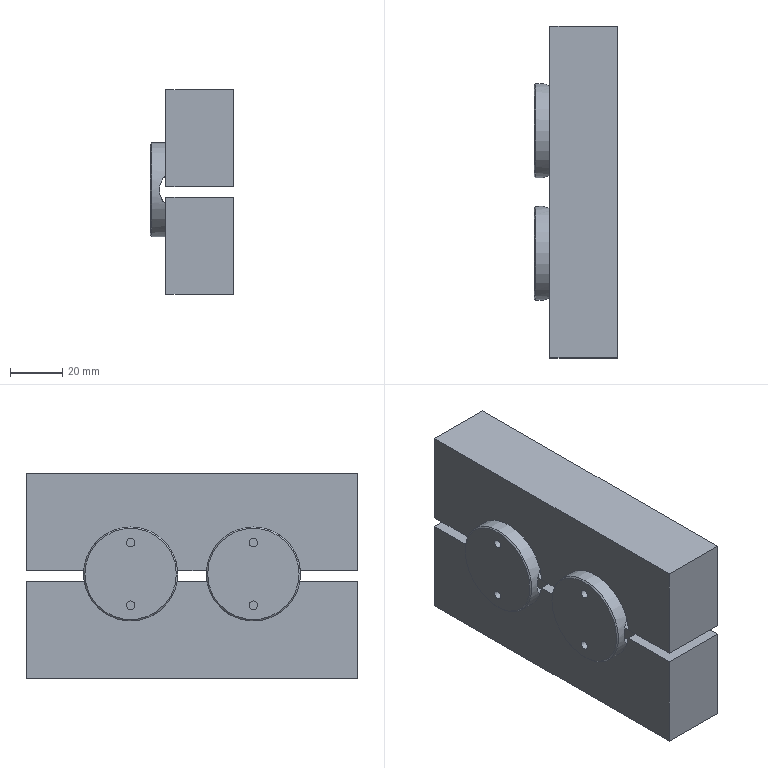Part | NX | 4 solids | 40 faces | box 32 x 127 x 78.432 mm | volume 253572 mm3 | plane 22 | cylinder 12 | cone 6 | commonest cylinder face diameters 36 x6 3.3 x4 15 x2
STEP:
#1=CARTESIAN_POINT('',(-169.277,51.261,125.416));
#2=VERTEX_POINT('',#1);
#3=CARTESIAN_POINT('',(-169.277,178.261,125.416));
#4=VERTEX_POINT('',#3);
#5=CARTESIAN_POINT('',(-169.277,114.761,125.416));
#6=DIRECTION('',(0.,1.,0.));
#7=VECTOR('',#6,1000.);
#8=LINE('',#5,#7);
#9=EDGE_CURVE('',#2,#4,#8,.T.);
#10=ORIENTED_EDGE('',*,*,#9,.T.);
#11=CARTESIAN_POINT('',(-169.277,178.261,162.632));
#12=VERTEX_POINT('',#11);
#13=CARTESIAN_POINT('',(-169.277,178.261,123.416));
#14=DIRECTION('',(0.,0.,-1.));
#15=VECTOR('',#14,1000.);
#16=LINE('',#13,#15);
#17=EDGE_CURVE('',#12,#4,#16,.T.);
#18=ORIENTED_EDGE('',*,*,#17,.F.);
#19=CARTESIAN_POINT('',(-169.277,51.261,162.632));
#20=VERTEX_POINT('',#19);
#21=CARTESIAN_POINT('',(-169.277,114.761,162.632));
#22=DIRECTION('',(0.,1.,0.));
#23=VECTOR('',#22,1000.);
#24=LINE('',#21,#23);
#25=EDGE_CURVE('',#20,#12,#24,.T.);
#26=ORIENTED_EDGE('',*,*,#25,.F.);
#27=CARTESIAN_POINT('',(-169.277,51.261,123.416));
#28=DIRECTION('',(0.,0.,1.));
#29=VECTOR('',#28,1000.);
#30=LINE('',#27,#29);
#31=EDGE_CURVE('',#2,#20,#30,.T.);
#32=ORIENTED_EDGE('',*,*,#31,.F.);
#33=EDGE_LOOP('',(#10,#18,#26,#32));
#34=FACE_BOUND('',#33,.T.);
#35=CARTESIAN_POINT('',(-169.277,114.761,123.416));
#36=DIRECTION('',(1.,0.,0.));
#37=DIRECTION('',(0.,0.,-1.));
#38=AXIS2_PLACEMENT_3D('',#35,#36,#37);
#39=PLANE('',#38);
#40=ADVANCED_FACE('',(#34),#39,.T.);
#41=CARTESIAN_POINT('',(-195.277,51.261,125.416));
#42=VERTEX_POINT('',#41);
#43=CARTESIAN_POINT('',(-199.777,51.261,125.416));
#44=DIRECTION('',(-1.,0.,0.));
#45=VECTOR('',#44,1000.);
#46=LINE('',#43,#45);
#47=EDGE_CURVE('',#2,#42,#46,.T.);
#48=ORIENTED_EDGE('',*,*,#47,.F.);
#49=ORIENTED_EDGE('',*,*,#31,.T.);
#50=CARTESIAN_POINT('',(-195.277,51.261,162.632));
#51=VERTEX_POINT('',#50);
#52=CARTESIAN_POINT('',(-199.777,51.261,162.632));
#53=DIRECTION('',(1.,0.,0.));
#54=VECTOR('',#53,1000.);
#55=LINE('',#52,#54);
#56=EDGE_CURVE('',#51,#20,#55,.T.);
#57=ORIENTED_EDGE('',*,*,#56,.F.);
#58=CARTESIAN_POINT('',(-195.277,51.261,123.416));
#59=DIRECTION('',(0.,0.,1.));
#60=VECTOR('',#59,1000.);
#61=LINE('',#58,#60);
#62=EDGE_CURVE('',#51,#42,#61,.F.);
#63=ORIENTED_EDGE('',*,*,#62,.T.);
#64=EDGE_LOOP('',(#48,#49,#57,#63));
#65=FACE_BOUND('',#64,.T.);
#66=CARTESIAN_POINT('',(-199.777,51.261,123.416));
#67=DIRECTION('',(0.,-1.,0.));
#68=DIRECTION('',(0.,0.,-1.));
#69=AXIS2_PLACEMENT_3D('',#66,#67,#68);
#70=PLANE('',#69);
#71=ADVANCED_FACE('',(#65),#70,.T.);
#72=ORIENTED_EDGE('',*,*,#56,.T.);
#73=ORIENTED_EDGE('',*,*,#25,.T.);
#74=CARTESIAN_POINT('',(-195.277,178.261,162.632));
#75=VERTEX_POINT('',#74);
#76=CARTESIAN_POINT('',(-199.777,178.261,162.632));
#77=DIRECTION('',(1.,0.,0.));
#78=VECTOR('',#77,1000.);
#79=LINE('',#76,#78);
#80=EDGE_CURVE('',#75,#12,#79,.T.);
#81=ORIENTED_EDGE('',*,*,#80,.F.);
#82=CARTESIAN_POINT('',(-195.277,114.761,162.632));
#83=DIRECTION('',(0.,1.,0.));
#84=VECTOR('',#83,1000.);
#85=LINE('',#82,#84);
#86=EDGE_CURVE('',#75,#51,#85,.F.);
#87=ORIENTED_EDGE('',*,*,#86,.T.);
#88=EDGE_LOOP('',(#72,#73,#81,#87));
#89=FACE_BOUND('',#88,.T.);
#90=CARTESIAN_POINT('',(-199.777,114.761,162.632));
#91=DIRECTION('',(0.,0.,1.));
#92=DIRECTION('',(1.,0.,0.));
#93=AXIS2_PLACEMENT_3D('',#90,#91,#92);
#94=PLANE('',#93);
#95=ADVANCED_FACE('',(#89),#94,.T.);
#96=CARTESIAN_POINT('',(-195.277,73.302,125.416));
#97=VERTEX_POINT('',#96);
#98=CARTESIAN_POINT('',(-195.277,114.761,125.416));
#99=DIRECTION('',(0.,1.,0.));
#100=VECTOR('',#99,1000.);
#101=LINE('',#98,#100);
#102=EDGE_CURVE('',#97,#42,#101,.F.);
#103=ORIENTED_EDGE('',*,*,#102,.T.);
#104=ORIENTED_EDGE('',*,*,#62,.F.);
#105=ORIENTED_EDGE('',*,*,#86,.F.);
#106=CARTESIAN_POINT('',(-195.277,178.261,125.416));
#107=VERTEX_POINT('',#106);
#108=CARTESIAN_POINT('',(-195.277,178.261,123.416));
#109=DIRECTION('',(0.,0.,-1.));
#110=VECTOR('',#109,1000.);
#111=LINE('',#108,#110);
#112=EDGE_CURVE('',#107,#75,#111,.F.);
#113=ORIENTED_EDGE('',*,*,#112,.F.);
#114=CARTESIAN_POINT('',(-195.277,156.22,125.416));
#115=VERTEX_POINT('',#114);
#116=CARTESIAN_POINT('',(-195.277,114.761,125.416));
#117=DIRECTION('',(0.,1.,0.));
#118=VECTOR('',#117,1000.);
#119=LINE('',#116,#118);
#120=EDGE_CURVE('',#107,#115,#119,.F.);
#121=ORIENTED_EDGE('',*,*,#120,.T.);
#122=CARTESIAN_POINT('',(-195.277,120.302,125.416));
#123=VERTEX_POINT('',#122);
#124=CARTESIAN_POINT('',(-195.277,138.261,124.2));
#125=DIRECTION('',(1.,0.,0.));
#126=DIRECTION('',(0.,1.,0.));
#127=AXIS2_PLACEMENT_3D('',#124,#125,#126);
#128=CIRCLE('',#127,18.);
#129=EDGE_CURVE('',#123,#115,#128,.F.);
#130=ORIENTED_EDGE('',*,*,#129,.F.);
#131=CARTESIAN_POINT('',(-195.277,109.22,125.416));
#132=VERTEX_POINT('',#131);
#133=CARTESIAN_POINT('',(-195.277,114.761,125.416));
#134=DIRECTION('',(0.,1.,0.));
#135=VECTOR('',#134,1000.);
#136=LINE('',#133,#135);
#137=EDGE_CURVE('',#123,#132,#136,.F.);
#138=ORIENTED_EDGE('',*,*,#137,.T.);
#139=CARTESIAN_POINT('',(-195.277,91.261,124.2));
#140=DIRECTION('',(1.,0.,0.));
#141=DIRECTION('',(0.,1.,0.));
#142=AXIS2_PLACEMENT_3D('',#139,#140,#141);
#143=CIRCLE('',#142,18.);
#144=EDGE_CURVE('',#97,#132,#143,.F.);
#145=ORIENTED_EDGE('',*,*,#144,.F.);
#146=EDGE_LOOP('',(#103,#104,#105,#113,#121,#130,#138,#145));
#147=FACE_BOUND('',#146,.T.);
#148=CARTESIAN_POINT('',(-195.277,91.261,124.2));
#149=DIRECTION('',(1.,0.,0.));
#150=DIRECTION('',(0.,1.,0.));
#151=AXIS2_PLACEMENT_3D('',#148,#149,#150);
#152=PLANE('',#151);
#153=ADVANCED_FACE('',(#147),#152,.F.);
#154=CARTESIAN_POINT('',(-199.777,178.261,125.416));
#155=DIRECTION('',(1.,0.,0.));
#156=VECTOR('',#155,1000.);
#157=LINE('',#154,#156);
#158=EDGE_CURVE('',#107,#4,#157,.T.);
#159=ORIENTED_EDGE('',*,*,#158,.F.);
#160=ORIENTED_EDGE('',*,*,#112,.T.);
#161=ORIENTED_EDGE('',*,*,#80,.T.);
#162=ORIENTED_EDGE('',*,*,#17,.T.);
#163=EDGE_LOOP('',(#159,#160,#161,#162));
#164=FACE_BOUND('',#163,.T.);
#165=CARTESIAN_POINT('',(-199.777,178.261,123.416));
#166=DIRECTION('',(0.,1.,0.));
#167=DIRECTION('',(0.,0.,1.));
#168=AXIS2_PLACEMENT_3D('',#165,#166,#167);
#169=PLANE('',#168);
#170=ADVANCED_FACE('',(#164),#169,.T.);
#171=ORIENTED_EDGE('',*,*,#129,.T.);
#172=CARTESIAN_POINT('',(-191.277,156.22,125.416));
#173=VERTEX_POINT('',#172);
#174=CARTESIAN_POINT('',(-191.777,156.22,125.416));
#175=DIRECTION('',(-1.,0.,0.));
#176=VECTOR('',#175,1000.);
#177=LINE('',#174,#176);
#178=EDGE_CURVE('',#173,#115,#177,.T.);
#179=ORIENTED_EDGE('',*,*,#178,.F.);
#180=CARTESIAN_POINT('',(-191.277,120.302,125.416));
#181=VERTEX_POINT('',#180);
#182=CARTESIAN_POINT('',(-191.277,138.261,124.2));
#183=DIRECTION('',(-1.,0.,0.));
#184=DIRECTION('',(0.,0.,1.));
#185=AXIS2_PLACEMENT_3D('',#182,#183,#184);
#186=CIRCLE('',#185,18.);
#187=EDGE_CURVE('',#173,#181,#186,.F.);
#188=ORIENTED_EDGE('',*,*,#187,.T.);
#189=CARTESIAN_POINT('',(-191.777,120.302,125.416));
#190=DIRECTION('',(-1.,0.,0.));
#191=VECTOR('',#190,1000.);
#192=LINE('',#189,#191);
#193=EDGE_CURVE('',#123,#181,#192,.F.);
#194=ORIENTED_EDGE('',*,*,#193,.F.);
#195=EDGE_LOOP('',(#171,#179,#188,#194));
#196=FACE_BOUND('',#195,.T.);
#197=CARTESIAN_POINT('',(-191.777,138.261,124.2));
#198=DIRECTION('',(-1.,0.,0.));
#199=DIRECTION('',(0.,0.,1.));
#200=AXIS2_PLACEMENT_3D('',#197,#198,#199);
#201=CYLINDRICAL_SURFACE('',#200,18.);
#202=ADVANCED_FACE('',(#196),#201,.F.);
#203=CARTESIAN_POINT('',(-191.277,138.261,125.416));
#204=DIRECTION('',(0.,1.,0.));
#205=VECTOR('',#204,1000.);
#206=LINE('',#203,#205);
#207=EDGE_CURVE('',#181,#173,#206,.T.);
#208=ORIENTED_EDGE('',*,*,#207,.F.);
#209=ORIENTED_EDGE('',*,*,#187,.F.);
#210=EDGE_LOOP('',(#208,#209));
#211=FACE_BOUND('',#210,.T.);
#212=CARTESIAN_POINT('',(-191.277,138.261,124.2));
#213=DIRECTION('',(-1.,0.,0.));
#214=DIRECTION('',(0.,0.,1.));
#215=AXIS2_PLACEMENT_3D('',#212,#213,#214);
#216=PLANE('',#215);
#217=ADVANCED_FACE('',(#211),#216,.T.);
#218=ORIENTED_EDGE('',*,*,#144,.T.);
#219=CARTESIAN_POINT('',(-191.277,109.22,125.416));
#220=VERTEX_POINT('',#219);
#221=CARTESIAN_POINT('',(-191.777,109.22,125.416));
#222=DIRECTION('',(-1.,0.,0.));
#223=VECTOR('',#222,1000.);
#224=LINE('',#221,#223);
#225=EDGE_CURVE('',#220,#132,#224,.T.);
#226=ORIENTED_EDGE('',*,*,#225,.F.);
#227=CARTESIAN_POINT('',(-191.277,73.302,125.416));
#228=VERTEX_POINT('',#227);
#229=CARTESIAN_POINT('',(-191.277,91.261,124.2));
#230=DIRECTION('',(-1.,0.,0.));
#231=DIRECTION('',(0.,0.,1.));
#232=AXIS2_PLACEMENT_3D('',#229,#230,#231);
#233=CIRCLE('',#232,18.);
#234=EDGE_CURVE('',#220,#228,#233,.F.);
#235=ORIENTED_EDGE('',*,*,#234,.T.);
#236=CARTESIAN_POINT('',(-191.777,73.302,125.416));
#237=DIRECTION('',(-1.,0.,0.));
#238=VECTOR('',#237,1000.);
#239=LINE('',#236,#238);
#240=EDGE_CURVE('',#97,#228,#239,.F.);
#241=ORIENTED_EDGE('',*,*,#240,.F.);
#242=EDGE_LOOP('',(#218,#226,#235,#241));
#243=FACE_BOUND('',#242,.T.);
#244=CARTESIAN_POINT('',(-191.777,91.261,124.2));
#245=DIRECTION('',(-1.,0.,0.));
#246=DIRECTION('',(0.,0.,1.));
#247=AXIS2_PLACEMENT_3D('',#244,#245,#246);
#248=CYLINDRICAL_SURFACE('',#247,18.);
#249=ADVANCED_FACE('',(#243),#248,.F.);
#250=CARTESIAN_POINT('',(-191.277,114.761,125.416));
#251=DIRECTION('',(0.,-1.,0.));
#252=VECTOR('',#251,1000.);
#253=LINE('',#250,#252);
#254=EDGE_CURVE('',#220,#228,#253,.T.);
#255=ORIENTED_EDGE('',*,*,#254,.T.);
#256=ORIENTED_EDGE('',*,*,#234,.F.);
#257=EDGE_LOOP('',(#255,#256));
#258=FACE_BOUND('',#257,.T.);
#259=CARTESIAN_POINT('',(-191.277,91.261,124.2));
#260=DIRECTION('',(-1.,0.,0.));
#261=DIRECTION('',(0.,0.,1.));
#262=AXIS2_PLACEMENT_3D('',#259,#260,#261);
#263=PLANE('',#262);
#264=ADVANCED_FACE('',(#258),#263,.T.);
#265=ORIENTED_EDGE('',*,*,#120,.F.);
#266=ORIENTED_EDGE('',*,*,#158,.T.);
#267=ORIENTED_EDGE('',*,*,#9,.F.);
#268=ORIENTED_EDGE('',*,*,#47,.T.);
#269=ORIENTED_EDGE('',*,*,#102,.F.);
#270=ORIENTED_EDGE('',*,*,#240,.T.);
#271=ORIENTED_EDGE('',*,*,#254,.F.);
#272=ORIENTED_EDGE('',*,*,#225,.T.);
#273=ORIENTED_EDGE('',*,*,#137,.F.);
#274=ORIENTED_EDGE('',*,*,#193,.T.);
#275=ORIENTED_EDGE('',*,*,#207,.T.);
#276=ORIENTED_EDGE('',*,*,#178,.T.);
#277=EDGE_LOOP('',(#265,#266,#267,#268,#269,#270,#271,#272,#273,#274,#275,#276));
#278=FACE_BOUND('',#277,.T.);
#279=CARTESIAN_POINT('',(-182.277,114.761,125.416));
#280=DIRECTION('',(0.,0.,1.));
#281=DIRECTION('',(1.,0.,0.));
#282=AXIS2_PLACEMENT_3D('',#279,#280,#281);
#283=PLANE('',#282);
#284=ADVANCED_FACE('',(#278),#283,.F.);
#285=CLOSED_SHELL('',(#40,#71,#95,#153,#170,#202,#217,#249,#264,#284));
#286=MANIFOLD_SOLID_BREP('',#285);
#287=CARTESIAN_POINT('',(-191.777,107.693,116.852));
#288=VERTEX_POINT('',#287);
#289=CARTESIAN_POINT('',(-191.277,107.104,116.767));
#290=VERTEX_POINT('',#289);
#291=CARTESIAN_POINT('',(-191.777,107.693,116.852));
#292=CARTESIAN_POINT('',(-191.611,107.496,116.818));
#293=CARTESIAN_POINT('',(-191.445,107.3,116.79));
#294=CARTESIAN_POINT('',(-191.277,107.104,116.767));
#295=B_SPLINE_CURVE_WITH_KNOTS('',3,(#291,#292,#293,#294),.UNSPECIFIED.,.F.,.F.,(4,4),(0.,1.),.UNSPECIFIED.);
#296=EDGE_CURVE('',#288,#290,#295,.T.);
#297=ORIENTED_EDGE('',*,*,#296,.T.);
#298=CARTESIAN_POINT('',(-191.277,75.418,116.767));
#299=VERTEX_POINT('',#298);
#300=CARTESIAN_POINT('',(-191.277,91.261,124.2));
#301=DIRECTION('',(1.,0.,0.));
#302=DIRECTION('',(0.,1.,0.));
#303=AXIS2_PLACEMENT_3D('',#300,#301,#302);
#304=CIRCLE('',#303,17.5);
#305=EDGE_CURVE('',#299,#290,#304,.T.);
#306=ORIENTED_EDGE('',*,*,#305,.F.);
#307=CARTESIAN_POINT('',(-191.777,74.829,116.852));
#308=VERTEX_POINT('',#307);
#309=CARTESIAN_POINT('',(-191.277,75.418,116.767));
#310=CARTESIAN_POINT('',(-191.445,75.222,116.79));
#311=CARTESIAN_POINT('',(-191.611,75.026,116.818));
#312=CARTESIAN_POINT('',(-191.777,74.829,116.852));
#313=B_SPLINE_CURVE_WITH_KNOTS('',3,(#309,#310,#311,#312),.UNSPECIFIED.,.F.,.F.,(4,4),(0.,1.),.UNSPECIFIED.);
#314=EDGE_CURVE('',#299,#308,#313,.T.);
#315=ORIENTED_EDGE('',*,*,#314,.T.);
#316=CARTESIAN_POINT('',(-191.777,91.261,124.2));
#317=DIRECTION('',(-1.,0.,0.));
#318=DIRECTION('',(0.,0.,-1.));
#319=AXIS2_PLACEMENT_3D('',#316,#317,#318);
#320=CIRCLE('',#319,18.);
#321=EDGE_CURVE('',#288,#308,#320,.T.);
#322=ORIENTED_EDGE('',*,*,#321,.F.);
#323=EDGE_LOOP('',(#297,#306,#315,#322));
#324=FACE_BOUND('',#323,.T.);
#325=CARTESIAN_POINT('',(-191.777,91.261,124.2));
#326=DIRECTION('',(-1.,0.,0.));
#327=DIRECTION('',(0.,1.,0.));
#328=AXIS2_PLACEMENT_3D('',#325,#326,#327);
#329=CONICAL_SURFACE('',#328,18.,0.7854);
#330=ADVANCED_FACE('',(#324),#329,.T.);
#331=CARTESIAN_POINT('',(-191.777,74.829,131.548));
#332=VERTEX_POINT('',#331);
#333=CARTESIAN_POINT('',(-191.277,75.418,131.633));
#334=VERTEX_POINT('',#333);
#335=CARTESIAN_POINT('',(-191.777,74.829,131.548));
#336=CARTESIAN_POINT('',(-191.611,75.026,131.582));
#337=CARTESIAN_POINT('',(-191.445,75.222,131.61));
#338=CARTESIAN_POINT('',(-191.277,75.418,131.633));
#339=B_SPLINE_CURVE_WITH_KNOTS('',3,(#335,#336,#337,#338),.UNSPECIFIED.,.F.,.F.,(4,4),(0.,1.),.UNSPECIFIED.);
#340=EDGE_CURVE('',#332,#334,#339,.T.);
#341=ORIENTED_EDGE('',*,*,#340,.T.);
#342=CARTESIAN_POINT('',(-191.277,107.104,131.633));
#343=VERTEX_POINT('',#342);
#344=CARTESIAN_POINT('',(-191.277,91.261,124.2));
#345=DIRECTION('',(1.,0.,0.));
#346=DIRECTION('',(0.,1.,0.));
#347=AXIS2_PLACEMENT_3D('',#344,#345,#346);
#348=CIRCLE('',#347,17.5);
#349=EDGE_CURVE('',#343,#334,#348,.T.);
#350=ORIENTED_EDGE('',*,*,#349,.F.);
#351=CARTESIAN_POINT('',(-191.777,107.693,131.548));
#352=VERTEX_POINT('',#351);
#353=CARTESIAN_POINT('',(-191.277,107.104,131.633));
#354=CARTESIAN_POINT('',(-191.445,107.3,131.61));
#355=CARTESIAN_POINT('',(-191.611,107.496,131.582));
#356=CARTESIAN_POINT('',(-191.777,107.693,131.548));
#357=B_SPLINE_CURVE_WITH_KNOTS('',3,(#353,#354,#355,#356),.UNSPECIFIED.,.F.,.F.,(4,4),(0.,1.),.UNSPECIFIED.);
#358=EDGE_CURVE('',#343,#352,#357,.T.);
#359=ORIENTED_EDGE('',*,*,#358,.T.);
#360=CARTESIAN_POINT('',(-191.777,91.261,124.2));
#361=DIRECTION('',(-1.,0.,0.));
#362=DIRECTION('',(0.,0.,-1.));
#363=AXIS2_PLACEMENT_3D('',#360,#361,#362);
#364=CIRCLE('',#363,18.);
#365=EDGE_CURVE('',#332,#352,#364,.T.);
#366=ORIENTED_EDGE('',*,*,#365,.F.);
#367=EDGE_LOOP('',(#341,#350,#359,#366));
#368=FACE_BOUND('',#367,.T.);
#369=CARTESIAN_POINT('',(-191.777,91.261,124.2));
#370=DIRECTION('',(-1.,0.,0.));
#371=DIRECTION('',(0.,1.,0.));
#372=AXIS2_PLACEMENT_3D('',#369,#370,#371);
#373=CONICAL_SURFACE('',#372,18.,0.7854);
#374=ADVANCED_FACE('',(#368),#373,.T.);
#375=CARTESIAN_POINT('',(-191.277,91.261,116.767));
#376=DIRECTION('',(0.,-1.,0.));
#377=VECTOR('',#376,1000.);
#378=LINE('',#375,#377);
#379=EDGE_CURVE('',#290,#299,#378,.T.);
#380=ORIENTED_EDGE('',*,*,#379,.T.);
#381=ORIENTED_EDGE('',*,*,#305,.T.);
#382=EDGE_LOOP('',(#380,#381));
#383=FACE_BOUND('',#382,.T.);
#384=CARTESIAN_POINT('',(-191.277,91.261,113.85));
#385=VERTEX_POINT('',#384);
#386=CARTESIAN_POINT('',(-191.277,91.261,112.2));
#387=DIRECTION('',(-1.,0.,0.));
#388=DIRECTION('',(0.,0.,1.));
#389=AXIS2_PLACEMENT_3D('',#386,#387,#388);
#390=CIRCLE('',#389,1.65);
#391=EDGE_CURVE('',#385,#385,#390,.T.);
#392=ORIENTED_EDGE('',*,*,#391,.T.);
#393=EDGE_LOOP('',(#392));
#394=FACE_BOUND('',#393,.T.);
#395=CARTESIAN_POINT('',(-191.277,91.261,124.2));
#396=DIRECTION('',(1.,0.,0.));
#397=DIRECTION('',(0.,0.,1.));
#398=AXIS2_PLACEMENT_3D('',#395,#396,#397);
#399=PLANE('',#398);
#400=ADVANCED_FACE('',(#383,#394),#399,.T.);
#401=CARTESIAN_POINT('',(-191.277,91.261,131.633));
#402=DIRECTION('',(0.,1.,0.));
#403=VECTOR('',#402,1000.);
#404=LINE('',#401,#403);
#405=EDGE_CURVE('',#334,#343,#404,.T.);
#406=ORIENTED_EDGE('',*,*,#405,.T.);
#407=ORIENTED_EDGE('',*,*,#349,.T.);
#408=EDGE_LOOP('',(#406,#407));
#409=FACE_BOUND('',#408,.T.);
#410=CARTESIAN_POINT('',(-191.277,91.261,137.85));
#411=VERTEX_POINT('',#410);
#412=CARTESIAN_POINT('',(-191.277,91.261,136.2));
#413=DIRECTION('',(-1.,0.,0.));
#414=DIRECTION('',(0.,0.,1.));
#415=AXIS2_PLACEMENT_3D('',#412,#413,#414);
#416=CIRCLE('',#415,1.65);
#417=EDGE_CURVE('',#411,#411,#416,.T.);
#418=ORIENTED_EDGE('',*,*,#417,.T.);
#419=EDGE_LOOP('',(#418));
#420=FACE_BOUND('',#419,.T.);
#421=CARTESIAN_POINT('',(-191.277,91.261,124.2));
#422=DIRECTION('',(1.,0.,0.));
#423=DIRECTION('',(0.,0.,1.));
#424=AXIS2_PLACEMENT_3D('',#421,#422,#423);
#425=PLANE('',#424);
#426=ADVANCED_FACE('',(#409,#420),#425,.T.);
#427=CARTESIAN_POINT('',(-201.277,91.261,137.85));
#428=VERTEX_POINT('',#427);
#429=CARTESIAN_POINT('',(-201.277,91.261,136.2));
#430=DIRECTION('',(-1.,0.,0.));
#431=DIRECTION('',(0.,0.,1.));
#432=AXIS2_PLACEMENT_3D('',#429,#430,#431);
#433=CIRCLE('',#432,1.65);
#434=EDGE_CURVE('',#428,#428,#433,.T.);
#435=ORIENTED_EDGE('',*,*,#434,.F.);
#436=EDGE_LOOP('',(#435));
#437=FACE_BOUND('',#436,.T.);
#438=CARTESIAN_POINT('',(-201.277,91.261,113.85));
#439=VERTEX_POINT('',#438);
#440=CARTESIAN_POINT('',(-201.277,91.261,112.2));
#441=DIRECTION('',(-1.,0.,0.));
#442=DIRECTION('',(0.,0.,1.));
#443=AXIS2_PLACEMENT_3D('',#440,#441,#442);
#444=CIRCLE('',#443,1.65);
#445=EDGE_CURVE('',#439,#439,#444,.T.);
#446=ORIENTED_EDGE('',*,*,#445,.F.);
#447=EDGE_LOOP('',(#446));
#448=FACE_BOUND('',#447,.T.);
#449=CARTESIAN_POINT('',(-201.277,73.761,124.2));
#450=VERTEX_POINT('',#449);
#451=CARTESIAN_POINT('',(-201.277,91.261,124.2));
#452=DIRECTION('',(1.,0.,0.));
#453=DIRECTION('',(0.,-1.,0.));
#454=AXIS2_PLACEMENT_3D('',#451,#452,#453);
#455=CIRCLE('',#454,17.5);
#456=EDGE_CURVE('',#450,#450,#455,.T.);
#457=ORIENTED_EDGE('',*,*,#456,.F.);
#458=EDGE_LOOP('',(#457));
#459=FACE_BOUND('',#458,.T.);
#460=CARTESIAN_POINT('',(-201.277,91.261,124.2));
#461=DIRECTION('',(1.,0.,0.));
#462=DIRECTION('',(0.,0.,1.));
#463=AXIS2_PLACEMENT_3D('',#460,#461,#462);
#464=PLANE('',#463);
#465=ADVANCED_FACE('',(#437,#448,#459),#464,.F.);
#466=ORIENTED_EDGE('',*,*,#434,.T.);
#467=EDGE_LOOP('',(#466));
#468=FACE_BOUND('',#467,.T.);
#469=ORIENTED_EDGE('',*,*,#417,.F.);
#470=EDGE_LOOP('',(#469));
#471=FACE_BOUND('',#470,.T.);
#472=CARTESIAN_POINT('',(-191.277,91.261,136.2));
#473=DIRECTION('',(1.,0.,0.));
#474=DIRECTION('',(0.,0.,1.));
#475=AXIS2_PLACEMENT_3D('',#472,#473,#474);
#476=CYLINDRICAL_SURFACE('',#475,1.65);
#477=ADVANCED_FACE('',(#468,#471),#476,.F.);
#478=ORIENTED_EDGE('',*,*,#445,.T.);
#479=EDGE_LOOP('',(#478));
#480=FACE_BOUND('',#479,.T.);
#481=ORIENTED_EDGE('',*,*,#391,.F.);
#482=EDGE_LOOP('',(#481));
#483=FACE_BOUND('',#482,.T.);
#484=CARTESIAN_POINT('',(-191.277,91.261,112.2));
#485=DIRECTION('',(1.,0.,0.));
#486=DIRECTION('',(0.,0.,1.));
#487=AXIS2_PLACEMENT_3D('',#484,#485,#486);
#488=CYLINDRICAL_SURFACE('',#487,1.65);
#489=ADVANCED_FACE('',(#480,#483),#488,.F.);
#490=ORIENTED_EDGE('',*,*,#456,.T.);
#491=EDGE_LOOP('',(#490));
#492=FACE_BOUND('',#491,.T.);
#493=CARTESIAN_POINT('',(-200.777,91.261,142.2));
#494=VERTEX_POINT('',#493);
#495=CARTESIAN_POINT('',(-200.777,91.261,124.2));
#496=DIRECTION('',(-1.,0.,0.));
#497=DIRECTION('',(0.,0.,1.));
#498=AXIS2_PLACEMENT_3D('',#495,#496,#497);
#499=CIRCLE('',#498,18.);
#500=EDGE_CURVE('',#494,#494,#499,.T.);
#501=ORIENTED_EDGE('',*,*,#500,.T.);
#502=EDGE_LOOP('',(#501));
#503=FACE_BOUND('',#502,.T.);
#504=CARTESIAN_POINT('',(-200.777,91.261,124.2));
#505=DIRECTION('',(1.,0.,0.));
#506=DIRECTION('',(0.,-1.,0.));
#507=AXIS2_PLACEMENT_3D('',#504,#505,#506);
#508=CONICAL_SURFACE('',#507,18.,0.7854);
#509=ADVANCED_FACE('',(#492,#503),#508,.T.);
#510=ORIENTED_EDGE('',*,*,#500,.F.);
#511=EDGE_LOOP('',(#510));
#512=FACE_BOUND('',#511,.T.);
#513=ORIENTED_EDGE('',*,*,#365,.T.);
#514=CARTESIAN_POINT('',(-191.777,107.693,131.548));
#515=CARTESIAN_POINT('',(-193.487,107.849,131.199));
#516=CARTESIAN_POINT('',(-196.519,108.688,129.35));
#517=CARTESIAN_POINT('',(-198.405,109.548,124.214));
#518=CARTESIAN_POINT('',(-196.519,108.688,119.042));
#519=CARTESIAN_POINT('',(-193.487,107.849,117.201));
#520=CARTESIAN_POINT('',(-191.777,107.693,116.852));
#521=B_SPLINE_CURVE_WITH_KNOTS('',3,(#514,#515,#516,#517,#518,#519,#520),.UNSPECIFIED.,.F.,.F.,(4,1,1,1,4),(-0.01037,-0.005188,-0.000007788,0.005172,0.01035),.UNSPECIFIED.);
#522=EDGE_CURVE('',#352,#288,#521,.T.);
#523=ORIENTED_EDGE('',*,*,#522,.T.);
#524=ORIENTED_EDGE('',*,*,#321,.T.);
#525=CARTESIAN_POINT('',(-191.777,74.829,116.852));
#526=CARTESIAN_POINT('',(-193.487,74.673,117.201));
#527=CARTESIAN_POINT('',(-196.519,73.835,119.05));
#528=CARTESIAN_POINT('',(-198.405,72.974,124.186));
#529=CARTESIAN_POINT('',(-196.519,73.835,129.358));
#530=CARTESIAN_POINT('',(-193.487,74.673,131.199));
#531=CARTESIAN_POINT('',(-191.777,74.829,131.548));
#532=B_SPLINE_CURVE_WITH_KNOTS('',3,(#525,#526,#527,#528,#529,#530,#531),.UNSPECIFIED.,.F.,.F.,(4,1,1,1,4),(0.,0.005177,0.01035,0.01553,0.02071),.UNSPECIFIED.);
#533=EDGE_CURVE('',#308,#332,#532,.T.);
#534=ORIENTED_EDGE('',*,*,#533,.T.);
#535=EDGE_LOOP('',(#513,#523,#524,#534));
#536=FACE_BOUND('',#535,.T.);
#537=CARTESIAN_POINT('',(-191.277,91.261,124.2));
#538=DIRECTION('',(-1.,0.,0.));
#539=DIRECTION('',(0.,0.,-1.));
#540=AXIS2_PLACEMENT_3D('',#537,#538,#539);
#541=CYLINDRICAL_SURFACE('',#540,18.);
#542=ADVANCED_FACE('',(#512,#536),#541,.T.);
#543=ORIENTED_EDGE('',*,*,#522,.F.);
#544=ORIENTED_EDGE('',*,*,#358,.F.);
#545=ORIENTED_EDGE('',*,*,#405,.F.);
#546=ORIENTED_EDGE('',*,*,#340,.F.);
#547=ORIENTED_EDGE('',*,*,#533,.F.);
#548=ORIENTED_EDGE('',*,*,#314,.F.);
#549=ORIENTED_EDGE('',*,*,#379,.F.);
#550=ORIENTED_EDGE('',*,*,#296,.F.);
#551=EDGE_LOOP('',(#543,#544,#545,#546,#547,#548,#549,#550));
#552=FACE_BOUND('',#551,.T.);
#553=CARTESIAN_POINT('',(-190.277,109.261,124.2));
#554=DIRECTION('',(0.,-1.,0.));
#555=DIRECTION('',(-1.,0.,0.));
#556=AXIS2_PLACEMENT_3D('',#553,#554,#555);
#557=CYLINDRICAL_SURFACE('',#556,7.5);
#558=ADVANCED_FACE('',(#552),#557,.F.);
#559=CLOSED_SHELL('',(#330,#374,#400,#426,#465,#477,#489,#509,#542,#558));
#560=MANIFOLD_SOLID_BREP('',#559);
#561=CARTESIAN_POINT('',(-195.277,156.045,121.416));
#562=VERTEX_POINT('',#561);
#563=CARTESIAN_POINT('',(-195.277,178.261,121.416));
#564=VERTEX_POINT('',#563);
#565=CARTESIAN_POINT('',(-195.277,91.261,121.416));
#566=DIRECTION('',(0.,-1.,0.));
#567=VECTOR('',#566,1000.);
#568=LINE('',#565,#567);
#569=EDGE_CURVE('',#562,#564,#568,.F.);
#570=ORIENTED_EDGE('',*,*,#569,.F.);
#571=CARTESIAN_POINT('',(-191.277,156.045,121.416));
#572=VERTEX_POINT('',#571);
#573=CARTESIAN_POINT('',(-195.277,156.045,121.416));
#574=DIRECTION('',(-1.,0.,0.));
#575=VECTOR('',#574,1000.);
#576=LINE('',#573,#575);
#577=EDGE_CURVE('',#562,#572,#576,.F.);
#578=ORIENTED_EDGE('',*,*,#577,.T.);
#579=CARTESIAN_POINT('',(-191.277,120.478,121.416));
#580=VERTEX_POINT('',#579);
#581=CARTESIAN_POINT('',(-191.277,114.761,121.416));
#582=DIRECTION('',(0.,-1.,0.));
#583=VECTOR('',#582,1000.);
#584=LINE('',#581,#583);
#585=EDGE_CURVE('',#572,#580,#584,.T.);
#586=ORIENTED_EDGE('',*,*,#585,.T.);
#587=CARTESIAN_POINT('',(-195.277,120.478,121.416));
#588=VERTEX_POINT('',#587);
#589=CARTESIAN_POINT('',(-191.777,120.478,121.416));
#590=DIRECTION('',(-1.,0.,0.));
#591=VECTOR('',#590,1000.);
#592=LINE('',#589,#591);
#593=EDGE_CURVE('',#580,#588,#592,.T.);
#594=ORIENTED_EDGE('',*,*,#593,.T.);
#595=CARTESIAN_POINT('',(-195.277,109.045,121.416));
#596=VERTEX_POINT('',#595);
#597=CARTESIAN_POINT('',(-195.277,91.261,121.416));
#598=DIRECTION('',(0.,-1.,0.));
#599=VECTOR('',#598,1000.);
#600=LINE('',#597,#599);
#601=EDGE_CURVE('',#596,#588,#600,.F.);
#602=ORIENTED_EDGE('',*,*,#601,.F.);
#603=CARTESIAN_POINT('',(-191.277,109.045,121.416));
#604=VERTEX_POINT('',#603);
#605=CARTESIAN_POINT('',(-191.777,109.045,121.416));
#606=DIRECTION('',(-1.,0.,0.));
#607=VECTOR('',#606,1000.);
#608=LINE('',#605,#607);
#609=EDGE_CURVE('',#596,#604,#608,.F.);
#610=ORIENTED_EDGE('',*,*,#609,.T.);
#611=CARTESIAN_POINT('',(-191.277,73.478,121.416));
#612=VERTEX_POINT('',#611);
#613=CARTESIAN_POINT('',(-191.277,91.261,121.416));
#614=DIRECTION('',(0.,1.,0.));
#615=VECTOR('',#614,1000.);
#616=LINE('',#613,#615);
#617=EDGE_CURVE('',#612,#604,#616,.T.);
#618=ORIENTED_EDGE('',*,*,#617,.F.);
#619=CARTESIAN_POINT('',(-195.277,73.478,121.416));
#620=VERTEX_POINT('',#619);
#621=CARTESIAN_POINT('',(-191.777,73.478,121.416));
#622=DIRECTION('',(-1.,0.,0.));
#623=VECTOR('',#622,1000.);
#624=LINE('',#621,#623);
#625=EDGE_CURVE('',#612,#620,#624,.T.);
#626=ORIENTED_EDGE('',*,*,#625,.T.);
#627=CARTESIAN_POINT('',(-195.277,51.261,121.416));
#628=VERTEX_POINT('',#627);
#629=CARTESIAN_POINT('',(-195.277,91.261,121.416));
#630=DIRECTION('',(0.,-1.,0.));
#631=VECTOR('',#630,1000.);
#632=LINE('',#629,#631);
#633=EDGE_CURVE('',#628,#620,#632,.F.);
#634=ORIENTED_EDGE('',*,*,#633,.F.);
#635=CARTESIAN_POINT('',(-169.277,51.261,121.416));
#636=VERTEX_POINT('',#635);
#637=CARTESIAN_POINT('',(-182.277,51.261,121.416));
#638=DIRECTION('',(1.,0.,0.));
#639=VECTOR('',#638,1000.);
#640=LINE('',#637,#639);
#641=EDGE_CURVE('',#628,#636,#640,.T.);
#642=ORIENTED_EDGE('',*,*,#641,.T.);
#643=CARTESIAN_POINT('',(-169.277,178.261,121.416));
#644=VERTEX_POINT('',#643);
#645=CARTESIAN_POINT('',(-169.277,114.761,121.416));
#646=DIRECTION('',(0.,-1.,0.));
#647=VECTOR('',#646,1000.);
#648=LINE('',#645,#647);
#649=EDGE_CURVE('',#644,#636,#648,.T.);
#650=ORIENTED_EDGE('',*,*,#649,.F.);
#651=CARTESIAN_POINT('',(-182.277,178.261,121.416));
#652=DIRECTION('',(-1.,0.,0.));
#653=VECTOR('',#652,1000.);
#654=LINE('',#651,#653);
#655=EDGE_CURVE('',#644,#564,#654,.T.);
#656=ORIENTED_EDGE('',*,*,#655,.T.);
#657=EDGE_LOOP('',(#570,#578,#586,#594,#602,#610,#618,#626,#634,#642,#650,#656));
#658=FACE_BOUND('',#657,.T.);
#659=CARTESIAN_POINT('',(-182.277,114.761,121.416));
#660=DIRECTION('',(0.,0.,1.));
#661=DIRECTION('',(1.,0.,0.));
#662=AXIS2_PLACEMENT_3D('',#659,#660,#661);
#663=PLANE('',#662);
#664=ADVANCED_FACE('',(#658),#663,.T.);
#665=CARTESIAN_POINT('',(-195.277,178.261,84.2));
#666=VERTEX_POINT('',#665);
#667=CARTESIAN_POINT('',(-169.277,178.261,84.2));
#668=VERTEX_POINT('',#667);
#669=CARTESIAN_POINT('',(-199.777,178.261,84.2));
#670=DIRECTION('',(1.,0.,0.));
#671=VECTOR('',#670,1000.);
#672=LINE('',#669,#671);
#673=EDGE_CURVE('',#666,#668,#672,.T.);
#674=ORIENTED_EDGE('',*,*,#673,.T.);
#675=CARTESIAN_POINT('',(-169.277,51.261,84.2));
#676=VERTEX_POINT('',#675);
#677=CARTESIAN_POINT('',(-169.277,114.761,84.2));
#678=DIRECTION('',(0.,-1.,0.));
#679=VECTOR('',#678,1000.);
#680=LINE('',#677,#679);
#681=EDGE_CURVE('',#668,#676,#680,.T.);
#682=ORIENTED_EDGE('',*,*,#681,.T.);
#683=CARTESIAN_POINT('',(-195.277,51.261,84.2));
#684=VERTEX_POINT('',#683);
#685=CARTESIAN_POINT('',(-199.777,51.261,84.2));
#686=DIRECTION('',(1.,0.,0.));
#687=VECTOR('',#686,1000.);
#688=LINE('',#685,#687);
#689=EDGE_CURVE('',#684,#676,#688,.T.);
#690=ORIENTED_EDGE('',*,*,#689,.F.);
#691=CARTESIAN_POINT('',(-195.277,114.761,84.2));
#692=DIRECTION('',(0.,-1.,0.));
#693=VECTOR('',#692,1000.);
#694=LINE('',#691,#693);
#695=EDGE_CURVE('',#684,#666,#694,.F.);
#696=ORIENTED_EDGE('',*,*,#695,.T.);
#697=EDGE_LOOP('',(#674,#682,#690,#696));
#698=FACE_BOUND('',#697,.T.);
#699=CARTESIAN_POINT('',(-199.777,114.761,84.2));
#700=DIRECTION('',(0.,0.,-1.));
#701=DIRECTION('',(-1.,0.,0.));
#702=AXIS2_PLACEMENT_3D('',#699,#700,#701);
#703=PLANE('',#702);
#704=ADVANCED_FACE('',(#698),#703,.T.);
#705=CARTESIAN_POINT('',(-195.277,178.261,123.416));
#706=DIRECTION('',(0.,0.,-1.));
#707=VECTOR('',#706,1000.);
#708=LINE('',#705,#707);
#709=EDGE_CURVE('',#666,#564,#708,.F.);
#710=ORIENTED_EDGE('',*,*,#709,.T.);
#711=ORIENTED_EDGE('',*,*,#655,.F.);
#712=CARTESIAN_POINT('',(-169.277,178.261,123.416));
#713=DIRECTION('',(0.,0.,-1.));
#714=VECTOR('',#713,1000.);
#715=LINE('',#712,#714);
#716=EDGE_CURVE('',#644,#668,#715,.T.);
#717=ORIENTED_EDGE('',*,*,#716,.T.);
#718=ORIENTED_EDGE('',*,*,#673,.F.);
#719=EDGE_LOOP('',(#710,#711,#717,#718));
#720=FACE_BOUND('',#719,.T.);
#721=CARTESIAN_POINT('',(-199.777,178.261,123.416));
#722=DIRECTION('',(0.,1.,0.));
#723=DIRECTION('',(0.,0.,1.));
#724=AXIS2_PLACEMENT_3D('',#721,#722,#723);
#725=PLANE('',#724);
#726=ADVANCED_FACE('',(#720),#725,.T.);
#727=CARTESIAN_POINT('',(-191.277,138.261,124.2));
#728=DIRECTION('',(-1.,0.,0.));
#729=DIRECTION('',(0.,0.,1.));
#730=AXIS2_PLACEMENT_3D('',#727,#728,#729);
#731=CIRCLE('',#730,18.);
#732=EDGE_CURVE('',#580,#572,#731,.F.);
#733=ORIENTED_EDGE('',*,*,#732,.F.);
#734=ORIENTED_EDGE('',*,*,#585,.F.);
#735=EDGE_LOOP('',(#733,#734));
#736=FACE_BOUND('',#735,.T.);
#737=CARTESIAN_POINT('',(-191.277,138.261,124.2));
#738=DIRECTION('',(-1.,0.,0.));
#739=DIRECTION('',(0.,0.,1.));
#740=AXIS2_PLACEMENT_3D('',#737,#738,#739);
#741=PLANE('',#740);
#742=ADVANCED_FACE('',(#736),#741,.T.);
#743=ORIENTED_EDGE('',*,*,#577,.F.);
#744=CARTESIAN_POINT('',(-195.277,138.261,124.2));
#745=DIRECTION('',(1.,0.,0.));
#746=DIRECTION('',(0.,1.,0.));
#747=AXIS2_PLACEMENT_3D('',#744,#745,#746);
#748=CIRCLE('',#747,18.);
#749=EDGE_CURVE('',#562,#588,#748,.F.);
#750=ORIENTED_EDGE('',*,*,#749,.T.);
#751=ORIENTED_EDGE('',*,*,#593,.F.);
#752=ORIENTED_EDGE('',*,*,#732,.T.);
#753=EDGE_LOOP('',(#743,#750,#751,#752));
#754=FACE_BOUND('',#753,.T.);
#755=CARTESIAN_POINT('',(-191.777,138.261,124.2));
#756=DIRECTION('',(-1.,0.,0.));
#757=DIRECTION('',(0.,0.,1.));
#758=AXIS2_PLACEMENT_3D('',#755,#756,#757);
#759=CYLINDRICAL_SURFACE('',#758,18.);
#760=ADVANCED_FACE('',(#754),#759,.F.);
#761=CARTESIAN_POINT('',(-191.277,91.261,124.2));
#762=DIRECTION('',(-1.,0.,0.));
#763=DIRECTION('',(0.,0.,1.));
#764=AXIS2_PLACEMENT_3D('',#761,#762,#763);
#765=CIRCLE('',#764,18.);
#766=EDGE_CURVE('',#612,#604,#765,.F.);
#767=ORIENTED_EDGE('',*,*,#766,.F.);
#768=ORIENTED_EDGE('',*,*,#617,.T.);
#769=EDGE_LOOP('',(#767,#768));
#770=FACE_BOUND('',#769,.T.);
#771=CARTESIAN_POINT('',(-191.277,91.261,124.2));
#772=DIRECTION('',(-1.,0.,0.));
#773=DIRECTION('',(0.,0.,1.));
#774=AXIS2_PLACEMENT_3D('',#771,#772,#773);
#775=PLANE('',#774);
#776=ADVANCED_FACE('',(#770),#775,.T.);
#777=ORIENTED_EDGE('',*,*,#609,.F.);
#778=CARTESIAN_POINT('',(-195.277,91.261,124.2));
#779=DIRECTION('',(1.,0.,0.));
#780=DIRECTION('',(0.,1.,0.));
#781=AXIS2_PLACEMENT_3D('',#778,#779,#780);
#782=CIRCLE('',#781,18.);
#783=EDGE_CURVE('',#596,#620,#782,.F.);
#784=ORIENTED_EDGE('',*,*,#783,.T.);
#785=ORIENTED_EDGE('',*,*,#625,.F.);
#786=ORIENTED_EDGE('',*,*,#766,.T.);
#787=EDGE_LOOP('',(#777,#784,#785,#786));
#788=FACE_BOUND('',#787,.T.);
#789=CARTESIAN_POINT('',(-191.777,91.261,124.2));
#790=DIRECTION('',(-1.,0.,0.));
#791=DIRECTION('',(0.,0.,1.));
#792=AXIS2_PLACEMENT_3D('',#789,#790,#791);
#793=CYLINDRICAL_SURFACE('',#792,18.);
#794=ADVANCED_FACE('',(#788),#793,.F.);
#795=CARTESIAN_POINT('',(-195.277,51.261,123.416));
#796=DIRECTION('',(0.,0.,1.));
#797=VECTOR('',#796,1000.);
#798=LINE('',#795,#797);
#799=EDGE_CURVE('',#628,#684,#798,.F.);
#800=ORIENTED_EDGE('',*,*,#799,.F.);
#801=ORIENTED_EDGE('',*,*,#633,.T.);
#802=ORIENTED_EDGE('',*,*,#783,.F.);
#803=ORIENTED_EDGE('',*,*,#601,.T.);
#804=ORIENTED_EDGE('',*,*,#749,.F.);
#805=ORIENTED_EDGE('',*,*,#569,.T.);
#806=ORIENTED_EDGE('',*,*,#709,.F.);
#807=ORIENTED_EDGE('',*,*,#695,.F.);
#808=EDGE_LOOP('',(#800,#801,#802,#803,#804,#805,#806,#807));
#809=FACE_BOUND('',#808,.T.);
#810=CARTESIAN_POINT('',(-195.277,91.261,124.2));
#811=DIRECTION('',(1.,0.,0.));
#812=DIRECTION('',(0.,1.,0.));
#813=AXIS2_PLACEMENT_3D('',#810,#811,#812);
#814=PLANE('',#813);
#815=ADVANCED_FACE('',(#809),#814,.F.);
#816=CARTESIAN_POINT('',(-169.277,51.261,123.416));
#817=DIRECTION('',(0.,0.,1.));
#818=VECTOR('',#817,1000.);
#819=LINE('',#816,#818);
#820=EDGE_CURVE('',#676,#636,#819,.T.);
#821=ORIENTED_EDGE('',*,*,#820,.T.);
#822=ORIENTED_EDGE('',*,*,#641,.F.);
#823=ORIENTED_EDGE('',*,*,#799,.T.);
#824=ORIENTED_EDGE('',*,*,#689,.T.);
#825=EDGE_LOOP('',(#821,#822,#823,#824));
#826=FACE_BOUND('',#825,.T.);
#827=CARTESIAN_POINT('',(-199.777,51.261,123.416));
#828=DIRECTION('',(0.,-1.,0.));
#829=DIRECTION('',(0.,0.,-1.));
#830=AXIS2_PLACEMENT_3D('',#827,#828,#829);
#831=PLANE('',#830);
#832=ADVANCED_FACE('',(#826),#831,.T.);
#833=ORIENTED_EDGE('',*,*,#716,.F.);
#834=ORIENTED_EDGE('',*,*,#649,.T.);
#835=ORIENTED_EDGE('',*,*,#820,.F.);
#836=ORIENTED_EDGE('',*,*,#681,.F.);
#837=EDGE_LOOP('',(#833,#834,#835,#836));
#838=FACE_BOUND('',#837,.T.);
#839=CARTESIAN_POINT('',(-169.277,114.761,123.416));
#840=DIRECTION('',(1.,0.,0.));
#841=DIRECTION('',(0.,0.,-1.));
#842=AXIS2_PLACEMENT_3D('',#839,#840,#841);
#843=PLANE('',#842);
#844=ADVANCED_FACE('',(#838),#843,.T.);
#845=CLOSED_SHELL('',(#664,#704,#726,#742,#760,#776,#794,#815,#832,#844));
#846=MANIFOLD_SOLID_BREP('',#845);
#847=CARTESIAN_POINT('',(-191.777,154.693,116.852));
#848=VERTEX_POINT('',#847);
#849=CARTESIAN_POINT('',(-191.277,154.104,116.767));
#850=VERTEX_POINT('',#849);
#851=CARTESIAN_POINT('',(-191.777,154.693,116.852));
#852=CARTESIAN_POINT('',(-191.611,154.496,116.818));
#853=CARTESIAN_POINT('',(-191.445,154.3,116.79));
#854=CARTESIAN_POINT('',(-191.277,154.104,116.767));
#855=B_SPLINE_CURVE_WITH_KNOTS('',3,(#851,#852,#853,#854),.UNSPECIFIED.,.F.,.F.,(4,4),(0.,1.),.UNSPECIFIED.);
#856=EDGE_CURVE('',#848,#850,#855,.T.);
#857=ORIENTED_EDGE('',*,*,#856,.T.);
#858=CARTESIAN_POINT('',(-191.277,122.418,116.767));
#859=VERTEX_POINT('',#858);
#860=CARTESIAN_POINT('',(-191.277,138.261,124.2));
#861=DIRECTION('',(1.,0.,0.));
#862=DIRECTION('',(0.,1.,0.));
#863=AXIS2_PLACEMENT_3D('',#860,#861,#862);
#864=CIRCLE('',#863,17.5);
#865=EDGE_CURVE('',#859,#850,#864,.T.);
#866=ORIENTED_EDGE('',*,*,#865,.F.);
#867=CARTESIAN_POINT('',(-191.777,121.829,116.852));
#868=VERTEX_POINT('',#867);
#869=CARTESIAN_POINT('',(-191.277,122.418,116.767));
#870=CARTESIAN_POINT('',(-191.445,122.222,116.79));
#871=CARTESIAN_POINT('',(-191.611,122.026,116.818));
#872=CARTESIAN_POINT('',(-191.777,121.829,116.852));
#873=B_SPLINE_CURVE_WITH_KNOTS('',3,(#869,#870,#871,#872),.UNSPECIFIED.,.F.,.F.,(4,4),(0.,1.),.UNSPECIFIED.);
#874=EDGE_CURVE('',#859,#868,#873,.T.);
#875=ORIENTED_EDGE('',*,*,#874,.T.);
#876=CARTESIAN_POINT('',(-191.777,138.261,124.2));
#877=DIRECTION('',(-1.,0.,0.));
#878=DIRECTION('',(0.,0.,-1.));
#879=AXIS2_PLACEMENT_3D('',#876,#877,#878);
#880=CIRCLE('',#879,18.);
#881=EDGE_CURVE('',#848,#868,#880,.T.);
#882=ORIENTED_EDGE('',*,*,#881,.F.);
#883=EDGE_LOOP('',(#857,#866,#875,#882));
#884=FACE_BOUND('',#883,.T.);
#885=CARTESIAN_POINT('',(-191.777,138.261,124.2));
#886=DIRECTION('',(-1.,0.,0.));
#887=DIRECTION('',(0.,1.,0.));
#888=AXIS2_PLACEMENT_3D('',#885,#886,#887);
#889=CONICAL_SURFACE('',#888,18.,0.7854);
#890=ADVANCED_FACE('',(#884),#889,.T.);
#891=CARTESIAN_POINT('',(-191.777,121.829,131.548));
#892=VERTEX_POINT('',#891);
#893=CARTESIAN_POINT('',(-191.277,122.418,131.633));
#894=VERTEX_POINT('',#893);
#895=CARTESIAN_POINT('',(-191.777,121.829,131.548));
#896=CARTESIAN_POINT('',(-191.611,122.026,131.582));
#897=CARTESIAN_POINT('',(-191.445,122.222,131.61));
#898=CARTESIAN_POINT('',(-191.277,122.418,131.633));
#899=B_SPLINE_CURVE_WITH_KNOTS('',3,(#895,#896,#897,#898),.UNSPECIFIED.,.F.,.F.,(4,4),(0.,1.),.UNSPECIFIED.);
#900=EDGE_CURVE('',#892,#894,#899,.T.);
#901=ORIENTED_EDGE('',*,*,#900,.T.);
#902=CARTESIAN_POINT('',(-191.277,154.104,131.633));
#903=VERTEX_POINT('',#902);
#904=CARTESIAN_POINT('',(-191.277,138.261,124.2));
#905=DIRECTION('',(1.,0.,0.));
#906=DIRECTION('',(0.,1.,0.));
#907=AXIS2_PLACEMENT_3D('',#904,#905,#906);
#908=CIRCLE('',#907,17.5);
#909=EDGE_CURVE('',#903,#894,#908,.T.);
#910=ORIENTED_EDGE('',*,*,#909,.F.);
#911=CARTESIAN_POINT('',(-191.777,154.693,131.548));
#912=VERTEX_POINT('',#911);
#913=CARTESIAN_POINT('',(-191.277,154.104,131.633));
#914=CARTESIAN_POINT('',(-191.445,154.3,131.61));
#915=CARTESIAN_POINT('',(-191.611,154.496,131.582));
#916=CARTESIAN_POINT('',(-191.777,154.693,131.548));
#917=B_SPLINE_CURVE_WITH_KNOTS('',3,(#913,#914,#915,#916),.UNSPECIFIED.,.F.,.F.,(4,4),(0.,1.),.UNSPECIFIED.);
#918=EDGE_CURVE('',#903,#912,#917,.T.);
#919=ORIENTED_EDGE('',*,*,#918,.T.);
#920=CARTESIAN_POINT('',(-191.777,138.261,124.2));
#921=DIRECTION('',(-1.,0.,0.));
#922=DIRECTION('',(0.,0.,-1.));
#923=AXIS2_PLACEMENT_3D('',#920,#921,#922);
#924=CIRCLE('',#923,18.);
#925=EDGE_CURVE('',#892,#912,#924,.T.);
#926=ORIENTED_EDGE('',*,*,#925,.F.);
#927=EDGE_LOOP('',(#901,#910,#919,#926));
#928=FACE_BOUND('',#927,.T.);
#929=CARTESIAN_POINT('',(-191.777,138.261,124.2));
#930=DIRECTION('',(-1.,0.,0.));
#931=DIRECTION('',(0.,1.,0.));
#932=AXIS2_PLACEMENT_3D('',#929,#930,#931);
#933=CONICAL_SURFACE('',#932,18.,0.7854);
#934=ADVANCED_FACE('',(#928),#933,.T.);
#935=CARTESIAN_POINT('',(-191.277,138.261,116.767));
#936=DIRECTION('',(0.,-1.,0.));
#937=VECTOR('',#936,1000.);
#938=LINE('',#935,#937);
#939=EDGE_CURVE('',#850,#859,#938,.T.);
#940=ORIENTED_EDGE('',*,*,#939,.T.);
#941=ORIENTED_EDGE('',*,*,#865,.T.);
#942=EDGE_LOOP('',(#940,#941));
#943=FACE_BOUND('',#942,.T.);
#944=CARTESIAN_POINT('',(-191.277,138.261,113.85));
#945=VERTEX_POINT('',#944);
#946=CARTESIAN_POINT('',(-191.277,138.261,112.2));
#947=DIRECTION('',(-1.,0.,0.));
#948=DIRECTION('',(0.,0.,1.));
#949=AXIS2_PLACEMENT_3D('',#946,#947,#948);
#950=CIRCLE('',#949,1.65);
#951=EDGE_CURVE('',#945,#945,#950,.T.);
#952=ORIENTED_EDGE('',*,*,#951,.T.);
#953=EDGE_LOOP('',(#952));
#954=FACE_BOUND('',#953,.T.);
#955=CARTESIAN_POINT('',(-191.277,138.261,124.2));
#956=DIRECTION('',(1.,0.,0.));
#957=DIRECTION('',(0.,0.,1.));
#958=AXIS2_PLACEMENT_3D('',#955,#956,#957);
#959=PLANE('',#958);
#960=ADVANCED_FACE('',(#943,#954),#959,.T.);
#961=CARTESIAN_POINT('',(-191.277,138.261,131.633));
#962=DIRECTION('',(0.,1.,0.));
#963=VECTOR('',#962,1000.);
#964=LINE('',#961,#963);
#965=EDGE_CURVE('',#894,#903,#964,.T.);
#966=ORIENTED_EDGE('',*,*,#965,.T.);
#967=ORIENTED_EDGE('',*,*,#909,.T.);
#968=EDGE_LOOP('',(#966,#967));
#969=FACE_BOUND('',#968,.T.);
#970=CARTESIAN_POINT('',(-191.277,138.261,137.85));
#971=VERTEX_POINT('',#970);
#972=CARTESIAN_POINT('',(-191.277,138.261,136.2));
#973=DIRECTION('',(-1.,0.,0.));
#974=DIRECTION('',(0.,0.,1.));
#975=AXIS2_PLACEMENT_3D('',#972,#973,#974);
#976=CIRCLE('',#975,1.65);
#977=EDGE_CURVE('',#971,#971,#976,.T.);
#978=ORIENTED_EDGE('',*,*,#977,.T.);
#979=EDGE_LOOP('',(#978));
#980=FACE_BOUND('',#979,.T.);
#981=CARTESIAN_POINT('',(-191.277,138.261,124.2));
#982=DIRECTION('',(1.,0.,0.));
#983=DIRECTION('',(0.,0.,1.));
#984=AXIS2_PLACEMENT_3D('',#981,#982,#983);
#985=PLANE('',#984);
#986=ADVANCED_FACE('',(#969,#980),#985,.T.);
#987=CARTESIAN_POINT('',(-201.277,138.261,137.85));
#988=VERTEX_POINT('',#987);
#989=CARTESIAN_POINT('',(-201.277,138.261,136.2));
#990=DIRECTION('',(-1.,0.,0.));
#991=DIRECTION('',(0.,0.,1.));
#992=AXIS2_PLACEMENT_3D('',#989,#990,#991);
#993=CIRCLE('',#992,1.65);
#994=EDGE_CURVE('',#988,#988,#993,.T.);
#995=ORIENTED_EDGE('',*,*,#994,.F.);
#996=EDGE_LOOP('',(#995));
#997=FACE_BOUND('',#996,.T.);
#998=CARTESIAN_POINT('',(-201.277,138.261,113.85));
#999=VERTEX_POINT('',#998);
#1000=CARTESIAN_POINT('',(-201.277,138.261,112.2));
#1001=DIRECTION('',(-1.,0.,0.));
#1002=DIRECTION('',(0.,0.,1.));
#1003=AXIS2_PLACEMENT_3D('',#1000,#1001,#1002);
#1004=CIRCLE('',#1003,1.65);
#1005=EDGE_CURVE('',#999,#999,#1004,.T.);
#1006=ORIENTED_EDGE('',*,*,#1005,.F.);
#1007=EDGE_LOOP('',(#1006));
#1008=FACE_BOUND('',#1007,.T.);
#1009=CARTESIAN_POINT('',(-201.277,120.761,124.2));
#1010=VERTEX_POINT('',#1009);
#1011=CARTESIAN_POINT('',(-201.277,138.261,124.2));
#1012=DIRECTION('',(1.,0.,0.));
#1013=DIRECTION('',(0.,-1.,0.));
#1014=AXIS2_PLACEMENT_3D('',#1011,#1012,#1013);
#1015=CIRCLE('',#1014,17.5);
#1016=EDGE_CURVE('',#1010,#1010,#1015,.T.);
#1017=ORIENTED_EDGE('',*,*,#1016,.F.);
#1018=EDGE_LOOP('',(#1017));
#1019=FACE_BOUND('',#1018,.T.);
#1020=CARTESIAN_POINT('',(-201.277,138.261,124.2));
#1021=DIRECTION('',(1.,0.,0.));
#1022=DIRECTION('',(0.,0.,1.));
#1023=AXIS2_PLACEMENT_3D('',#1020,#1021,#1022);
#1024=PLANE('',#1023);
#1025=ADVANCED_FACE('',(#997,#1008,#1019),#1024,.F.);
#1026=ORIENTED_EDGE('',*,*,#994,.T.);
#1027=EDGE_LOOP('',(#1026));
#1028=FACE_BOUND('',#1027,.T.);
#1029=ORIENTED_EDGE('',*,*,#977,.F.);
#1030=EDGE_LOOP('',(#1029));
#1031=FACE_BOUND('',#1030,.T.);
#1032=CARTESIAN_POINT('',(-191.277,138.261,136.2));
#1033=DIRECTION('',(1.,0.,0.));
#1034=DIRECTION('',(0.,0.,1.));
#1035=AXIS2_PLACEMENT_3D('',#1032,#1033,#1034);
#1036=CYLINDRICAL_SURFACE('',#1035,1.65);
#1037=ADVANCED_FACE('',(#1028,#1031),#1036,.F.);
#1038=ORIENTED_EDGE('',*,*,#1005,.T.);
#1039=EDGE_LOOP('',(#1038));
#1040=FACE_BOUND('',#1039,.T.);
#1041=ORIENTED_EDGE('',*,*,#951,.F.);
#1042=EDGE_LOOP('',(#1041));
#1043=FACE_BOUND('',#1042,.T.);
#1044=CARTESIAN_POINT('',(-191.277,138.261,112.2));
#1045=DIRECTION('',(1.,0.,0.));
#1046=DIRECTION('',(0.,0.,1.));
#1047=AXIS2_PLACEMENT_3D('',#1044,#1045,#1046);
#1048=CYLINDRICAL_SURFACE('',#1047,1.65);
#1049=ADVANCED_FACE('',(#1040,#1043),#1048,.F.);
#1050=ORIENTED_EDGE('',*,*,#1016,.T.);
#1051=EDGE_LOOP('',(#1050));
#1052=FACE_BOUND('',#1051,.T.);
#1053=CARTESIAN_POINT('',(-200.777,138.261,142.2));
#1054=VERTEX_POINT('',#1053);
#1055=CARTESIAN_POINT('',(-200.777,138.261,124.2));
#1056=DIRECTION('',(-1.,0.,0.));
#1057=DIRECTION('',(0.,0.,1.));
#1058=AXIS2_PLACEMENT_3D('',#1055,#1056,#1057);
#1059=CIRCLE('',#1058,18.);
#1060=EDGE_CURVE('',#1054,#1054,#1059,.T.);
#1061=ORIENTED_EDGE('',*,*,#1060,.T.);
#1062=EDGE_LOOP('',(#1061));
#1063=FACE_BOUND('',#1062,.T.);
#1064=CARTESIAN_POINT('',(-200.777,138.261,124.2));
#1065=DIRECTION('',(1.,0.,0.));
#1066=DIRECTION('',(0.,-1.,0.));
#1067=AXIS2_PLACEMENT_3D('',#1064,#1065,#1066);
#1068=CONICAL_SURFACE('',#1067,18.,0.7854);
#1069=ADVANCED_FACE('',(#1052,#1063),#1068,.T.);
#1070=ORIENTED_EDGE('',*,*,#1060,.F.);
#1071=EDGE_LOOP('',(#1070));
#1072=FACE_BOUND('',#1071,.T.);
#1073=ORIENTED_EDGE('',*,*,#925,.T.);
#1074=CARTESIAN_POINT('',(-191.777,154.693,131.548));
#1075=CARTESIAN_POINT('',(-193.487,154.849,131.199));
#1076=CARTESIAN_POINT('',(-196.519,155.688,129.35));
#1077=CARTESIAN_POINT('',(-198.405,156.548,124.214));
#1078=CARTESIAN_POINT('',(-196.519,155.688,119.042));
#1079=CARTESIAN_POINT('',(-193.487,154.849,117.201));
#1080=CARTESIAN_POINT('',(-191.777,154.693,116.852));
#1081=B_SPLINE_CURVE_WITH_KNOTS('',3,(#1074,#1075,#1076,#1077,#1078,#1079,#1080),.UNSPECIFIED.,.F.,.F.,(4,1,1,1,4),(-0.01037,-0.005188,-0.000007788,0.005172,0.01035),.UNSPECIFIED.);
#1082=EDGE_CURVE('',#912,#848,#1081,.T.);
#1083=ORIENTED_EDGE('',*,*,#1082,.T.);
#1084=ORIENTED_EDGE('',*,*,#881,.T.);
#1085=CARTESIAN_POINT('',(-191.777,121.829,116.852));
#1086=CARTESIAN_POINT('',(-193.487,121.673,117.201));
#1087=CARTESIAN_POINT('',(-196.519,120.835,119.05));
#1088=CARTESIAN_POINT('',(-198.405,119.974,124.186));
#1089=CARTESIAN_POINT('',(-196.519,120.835,129.358));
#1090=CARTESIAN_POINT('',(-193.487,121.673,131.199));
#1091=CARTESIAN_POINT('',(-191.777,121.829,131.548));
#1092=B_SPLINE_CURVE_WITH_KNOTS('',3,(#1085,#1086,#1087,#1088,#1089,#1090,#1091),.UNSPECIFIED.,.F.,.F.,(4,1,1,1,4),(0.,0.005177,0.01035,0.01553,0.02071),.UNSPECIFIED.);
#1093=EDGE_CURVE('',#868,#892,#1092,.T.);
#1094=ORIENTED_EDGE('',*,*,#1093,.T.);
#1095=EDGE_LOOP('',(#1073,#1083,#1084,#1094));
#1096=FACE_BOUND('',#1095,.T.);
#1097=CARTESIAN_POINT('',(-191.277,138.261,124.2));
#1098=DIRECTION('',(-1.,0.,0.));
#1099=DIRECTION('',(0.,0.,-1.));
#1100=AXIS2_PLACEMENT_3D('',#1097,#1098,#1099);
#1101=CYLINDRICAL_SURFACE('',#1100,18.);
#1102=ADVANCED_FACE('',(#1072,#1096),#1101,.T.);
#1103=ORIENTED_EDGE('',*,*,#1082,.F.);
#1104=ORIENTED_EDGE('',*,*,#918,.F.);
#1105=ORIENTED_EDGE('',*,*,#965,.F.);
#1106=ORIENTED_EDGE('',*,*,#900,.F.);
#1107=ORIENTED_EDGE('',*,*,#1093,.F.);
#1108=ORIENTED_EDGE('',*,*,#874,.F.);
#1109=ORIENTED_EDGE('',*,*,#939,.F.);
#1110=ORIENTED_EDGE('',*,*,#856,.F.);
#1111=EDGE_LOOP('',(#1103,#1104,#1105,#1106,#1107,#1108,#1109,#1110));
#1112=FACE_BOUND('',#1111,.T.);
#1113=CARTESIAN_POINT('',(-190.277,156.261,124.2));
#1114=DIRECTION('',(0.,-1.,0.));
#1115=DIRECTION('',(-1.,0.,0.));
#1116=AXIS2_PLACEMENT_3D('',#1113,#1114,#1115);
#1117=CYLINDRICAL_SURFACE('',#1116,7.5);
#1118=ADVANCED_FACE('',(#1112),#1117,.F.);
#1119=CLOSED_SHELL('',(#890,#934,#960,#986,#1025,#1037,#1049,#1069,#1102,#1118));
#1120=MANIFOLD_SOLID_BREP('',#1119);
#1121=(LENGTH_UNIT()NAMED_UNIT(*)SI_UNIT(.MILLI.,.METRE.));
#1122=UNCERTAINTY_MEASURE_WITH_UNIT(LENGTH_MEASURE(0.0508),#1121,'','');
#1123=(NAMED_UNIT(*)PLANE_ANGLE_UNIT()SI_UNIT($,.RADIAN.));
#1124=(NAMED_UNIT(*)SI_UNIT($,.STERADIAN.)SOLID_ANGLE_UNIT());
#1125=(GEOMETRIC_REPRESENTATION_CONTEXT(3)GLOBAL_UNCERTAINTY_ASSIGNED_CONTEXT((#1122))GLOBAL_UNIT_ASSIGNED_CONTEXT((#1121,#1123,#1124))REPRESENTATION_CONTEXT('',''));
#1126=ADVANCED_BREP_SHAPE_REPRESENTATION('',(#286,#560,#846,#1120),#1125);